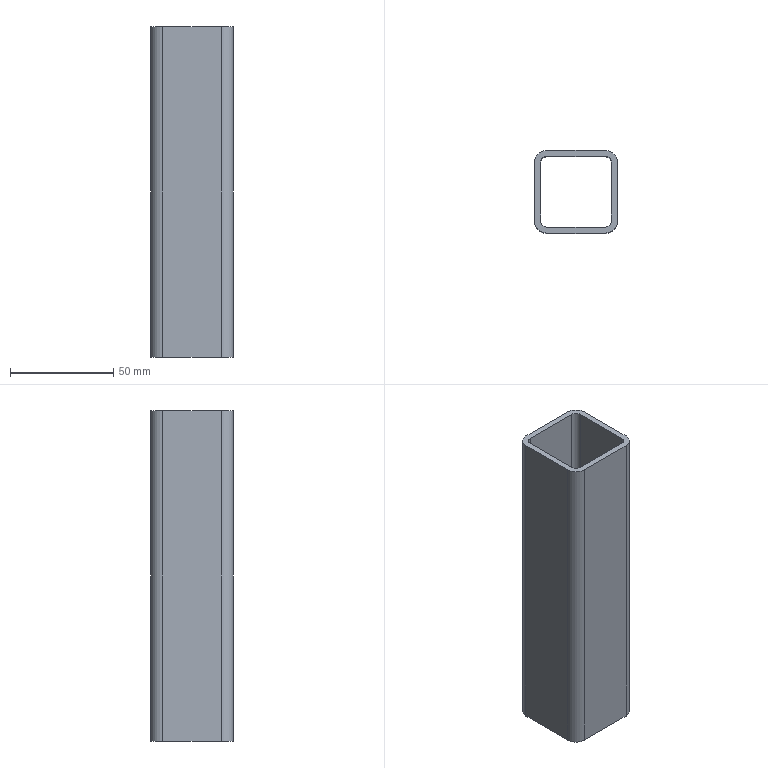Part | STEP file | DIN 59 410 - 40x40x2.9-200 | 1 solid | 18 faces | box 40 x 40 x 160 mm | volume 65392 mm3 | plane 10 | cylinder 8 | commonest cylinder face diameters 5.8 x4 11.6 x4
STEP:
#1=CARTESIAN_POINT('',(0.,0.,0.));
#2=DIRECTION('',(0.,0.,1.));
#3=DIRECTION('',(1.,0.,0.));
#4=AXIS2_PLACEMENT_3D('',#1,#2,#3);
#5=CARTESIAN_POINT('',(-14.2,-17.1,160.));
#6=VERTEX_POINT('',#5);
#7=CARTESIAN_POINT('',(14.2,-17.1,160.));
#8=VERTEX_POINT('',#7);
#9=CARTESIAN_POINT('',(7.1,-17.1,160.));
#10=DIRECTION('',(1.,0.,0.));
#11=VECTOR('',#10,1.);
#12=LINE('',#9,#11);
#13=CARTESIAN_POINT('',(14.2,-17.1,0.));
#14=DIRECTION('',(0.,-1.,0.));
#15=DIRECTION('',(0.,0.,-1.));
#16=AXIS2_PLACEMENT_3D('',#13,#14,#15);
#17=PLANE('',#16);
#18=CARTESIAN_POINT('',(-160.,-7.1));
#19=DIRECTION('',(0.,1.));
#20=VECTOR('',#19,1.);
#21=LINE('',#18,#20);
#22=(GEOMETRIC_REPRESENTATION_CONTEXT(2)PARAMETRIC_REPRESENTATION_CONTEXT()REPRESENTATION_CONTEXT('',''));
#23=DEFINITIONAL_REPRESENTATION('',(#21),#22);
#24=PCURVE('',#17,#23);
#25=CARTESIAN_POINT('',(0.,0.,160.));
#26=DIRECTION('',(0.,0.,1.));
#27=DIRECTION('',(1.,0.,0.));
#28=AXIS2_PLACEMENT_3D('',#25,#26,#27);
#29=PLANE('',#28);
#30=CARTESIAN_POINT('',(7.1,-17.1));
#31=DIRECTION('',(1.,0.));
#32=VECTOR('',#31,1.);
#33=LINE('',#30,#32);
#34=(GEOMETRIC_REPRESENTATION_CONTEXT(2)PARAMETRIC_REPRESENTATION_CONTEXT()REPRESENTATION_CONTEXT('',''));
#35=DEFINITIONAL_REPRESENTATION('',(#33),#34);
#36=PCURVE('',#29,#35);
#37=SURFACE_CURVE('',#12,(#24,#36),.PCURVE_S1.);
#38=EDGE_CURVE('',#6,#8,#37,.T.);
#39=ORIENTED_EDGE('',*,*,#38,.T.);
#40=CARTESIAN_POINT('',(14.2,-17.1,0.));
#41=VERTEX_POINT('',#40);
#42=CARTESIAN_POINT('',(14.2,-17.1,0.));
#43=DIRECTION('',(0.,0.,1.));
#44=VECTOR('',#43,1.);
#45=LINE('',#42,#44);
#46=CARTESIAN_POINT('',(0.,0.));
#47=DIRECTION('',(-1.,0.));
#48=VECTOR('',#47,1.);
#49=LINE('',#46,#48);
#50=(GEOMETRIC_REPRESENTATION_CONTEXT(2)PARAMETRIC_REPRESENTATION_CONTEXT()REPRESENTATION_CONTEXT('',''));
#51=DEFINITIONAL_REPRESENTATION('',(#49),#50);
#52=PCURVE('',#17,#51);
#53=CARTESIAN_POINT('',(14.2,-14.2,0.));
#54=DIRECTION('',(0.,0.,1.));
#55=DIRECTION('',(0.,1.,0.));
#56=AXIS2_PLACEMENT_3D('',#53,#54,#55);
#57=CYLINDRICAL_SURFACE('',#56,2.9);
#58=CARTESIAN_POINT('',(3.142,0.));
#59=DIRECTION('',(0.,1.));
#60=VECTOR('',#59,1.);
#61=LINE('',#58,#60);
#62=(GEOMETRIC_REPRESENTATION_CONTEXT(2)PARAMETRIC_REPRESENTATION_CONTEXT()REPRESENTATION_CONTEXT('',''));
#63=DEFINITIONAL_REPRESENTATION('',(#61),#62);
#64=PCURVE('',#57,#63);
#65=SURFACE_CURVE('',#45,(#52,#64),.PCURVE_S1.);
#66=EDGE_CURVE('',#41,#8,#65,.T.);
#67=ORIENTED_EDGE('',*,*,#66,.F.);
#68=CARTESIAN_POINT('',(-14.2,-17.1,0.));
#69=VERTEX_POINT('',#68);
#70=CARTESIAN_POINT('',(7.1,-17.1,0.));
#71=DIRECTION('',(1.,0.,0.));
#72=VECTOR('',#71,1.);
#73=LINE('',#70,#72);
#74=CARTESIAN_POINT('',(0.,-7.1));
#75=DIRECTION('',(0.,1.));
#76=VECTOR('',#75,1.);
#77=LINE('',#74,#76);
#78=(GEOMETRIC_REPRESENTATION_CONTEXT(2)PARAMETRIC_REPRESENTATION_CONTEXT()REPRESENTATION_CONTEXT('',''));
#79=DEFINITIONAL_REPRESENTATION('',(#77),#78);
#80=PCURVE('',#17,#79);
#81=CARTESIAN_POINT('',(0.,0.,0.));
#82=DIRECTION('',(0.,0.,1.));
#83=DIRECTION('',(1.,0.,0.));
#84=AXIS2_PLACEMENT_3D('',#81,#82,#83);
#85=PLANE('',#84);
#86=CARTESIAN_POINT('',(7.1,-17.1));
#87=DIRECTION('',(1.,0.));
#88=VECTOR('',#87,1.);
#89=LINE('',#86,#88);
#90=(GEOMETRIC_REPRESENTATION_CONTEXT(2)PARAMETRIC_REPRESENTATION_CONTEXT()REPRESENTATION_CONTEXT('',''));
#91=DEFINITIONAL_REPRESENTATION('',(#89),#90);
#92=PCURVE('',#85,#91);
#93=SURFACE_CURVE('',#73,(#80,#92),.PCURVE_S1.);
#94=EDGE_CURVE('',#69,#41,#93,.T.);
#95=ORIENTED_EDGE('',*,*,#94,.F.);
#96=CARTESIAN_POINT('',(-14.2,-17.1,0.));
#97=DIRECTION('',(0.,0.,1.));
#98=VECTOR('',#97,1.);
#99=LINE('',#96,#98);
#100=CARTESIAN_POINT('',(0.,-28.4));
#101=DIRECTION('',(-1.,0.));
#102=VECTOR('',#101,1.);
#103=LINE('',#100,#102);
#104=(GEOMETRIC_REPRESENTATION_CONTEXT(2)PARAMETRIC_REPRESENTATION_CONTEXT()REPRESENTATION_CONTEXT('',''));
#105=DEFINITIONAL_REPRESENTATION('',(#103),#104);
#106=PCURVE('',#17,#105);
#107=CARTESIAN_POINT('',(-14.2,-14.2,0.));
#108=DIRECTION('',(0.,0.,1.));
#109=DIRECTION('',(1.,0.,0.));
#110=AXIS2_PLACEMENT_3D('',#107,#108,#109);
#111=CYLINDRICAL_SURFACE('',#110,2.9);
#112=CARTESIAN_POINT('',(4.712,0.));
#113=DIRECTION('',(0.,1.));
#114=VECTOR('',#113,1.);
#115=LINE('',#112,#114);
#116=(GEOMETRIC_REPRESENTATION_CONTEXT(2)PARAMETRIC_REPRESENTATION_CONTEXT()REPRESENTATION_CONTEXT('',''));
#117=DEFINITIONAL_REPRESENTATION('',(#115),#116);
#118=PCURVE('',#111,#117);
#119=SURFACE_CURVE('',#99,(#106,#118),.PCURVE_S1.);
#120=EDGE_CURVE('',#69,#6,#119,.T.);
#121=ORIENTED_EDGE('',*,*,#120,.T.);
#122=EDGE_LOOP('',(#39,#67,#95,#121));
#123=FACE_BOUND('',#122,.T.);
#124=ADVANCED_FACE('',(#123),#17,.F.);
#125=ORIENTED_EDGE('',*,*,#66,.F.);
#126=CARTESIAN_POINT('',(17.1,-14.2,0.));
#127=VERTEX_POINT('',#126);
#128=CARTESIAN_POINT('',(14.2,-14.2,0.));
#129=DIRECTION('',(0.,0.,1.));
#130=DIRECTION('',(0.,1.,0.));
#131=AXIS2_PLACEMENT_3D('',#128,#129,#130);
#132=CIRCLE('',#131,2.9);
#133=CARTESIAN_POINT('',(0.,0.));
#134=DIRECTION('',(1.,0.));
#135=VECTOR('',#134,1.);
#136=LINE('',#133,#135);
#137=(GEOMETRIC_REPRESENTATION_CONTEXT(2)PARAMETRIC_REPRESENTATION_CONTEXT()REPRESENTATION_CONTEXT('',''));
#138=DEFINITIONAL_REPRESENTATION('',(#136),#137);
#139=PCURVE('',#57,#138);
#140=CARTESIAN_POINT('',(14.2,-14.2));
#141=DIRECTION('',(0.,1.));
#142=AXIS2_PLACEMENT_2D('',#140,#141);
#143=CIRCLE('',#142,2.9);
#144=(GEOMETRIC_REPRESENTATION_CONTEXT(2)PARAMETRIC_REPRESENTATION_CONTEXT()REPRESENTATION_CONTEXT('',''));
#145=DEFINITIONAL_REPRESENTATION('',(#143),#144);
#146=PCURVE('',#85,#145);
#147=SURFACE_CURVE('',#132,(#139,#146),.PCURVE_S1.);
#148=EDGE_CURVE('',#41,#127,#147,.T.);
#149=ORIENTED_EDGE('',*,*,#148,.T.);
#150=CARTESIAN_POINT('',(17.1,-14.2,160.));
#151=VERTEX_POINT('',#150);
#152=CARTESIAN_POINT('',(17.1,-14.2,0.));
#153=DIRECTION('',(0.,0.,1.));
#154=VECTOR('',#153,1.);
#155=LINE('',#152,#154);
#156=CARTESIAN_POINT('',(4.712,0.));
#157=DIRECTION('',(0.,1.));
#158=VECTOR('',#157,1.);
#159=LINE('',#156,#158);
#160=(GEOMETRIC_REPRESENTATION_CONTEXT(2)PARAMETRIC_REPRESENTATION_CONTEXT()REPRESENTATION_CONTEXT('',''));
#161=DEFINITIONAL_REPRESENTATION('',(#159),#160);
#162=PCURVE('',#57,#161);
#163=CARTESIAN_POINT('',(17.1,14.2,0.));
#164=DIRECTION('',(1.,0.,0.));
#165=DIRECTION('',(0.,0.,-1.));
#166=AXIS2_PLACEMENT_3D('',#163,#164,#165);
#167=PLANE('',#166);
#168=CARTESIAN_POINT('',(0.,-28.4));
#169=DIRECTION('',(-1.,0.));
#170=VECTOR('',#169,1.);
#171=LINE('',#168,#170);
#172=(GEOMETRIC_REPRESENTATION_CONTEXT(2)PARAMETRIC_REPRESENTATION_CONTEXT()REPRESENTATION_CONTEXT('',''));
#173=DEFINITIONAL_REPRESENTATION('',(#171),#172);
#174=PCURVE('',#167,#173);
#175=SURFACE_CURVE('',#155,(#162,#174),.PCURVE_S1.);
#176=EDGE_CURVE('',#127,#151,#175,.T.);
#177=ORIENTED_EDGE('',*,*,#176,.T.);
#178=CARTESIAN_POINT('',(14.2,-14.2,160.));
#179=DIRECTION('',(0.,0.,1.));
#180=DIRECTION('',(0.,1.,0.));
#181=AXIS2_PLACEMENT_3D('',#178,#179,#180);
#182=CIRCLE('',#181,2.9);
#183=CARTESIAN_POINT('',(0.,160.));
#184=DIRECTION('',(1.,0.));
#185=VECTOR('',#184,1.);
#186=LINE('',#183,#185);
#187=(GEOMETRIC_REPRESENTATION_CONTEXT(2)PARAMETRIC_REPRESENTATION_CONTEXT()REPRESENTATION_CONTEXT('',''));
#188=DEFINITIONAL_REPRESENTATION('',(#186),#187);
#189=PCURVE('',#57,#188);
#190=CARTESIAN_POINT('',(14.2,-14.2));
#191=DIRECTION('',(0.,1.));
#192=AXIS2_PLACEMENT_2D('',#190,#191);
#193=CIRCLE('',#192,2.9);
#194=(GEOMETRIC_REPRESENTATION_CONTEXT(2)PARAMETRIC_REPRESENTATION_CONTEXT()REPRESENTATION_CONTEXT('',''));
#195=DEFINITIONAL_REPRESENTATION('',(#193),#194);
#196=PCURVE('',#29,#195);
#197=SURFACE_CURVE('',#182,(#189,#196),.PCURVE_S1.);
#198=EDGE_CURVE('',#8,#151,#197,.T.);
#199=ORIENTED_EDGE('',*,*,#198,.F.);
#200=EDGE_LOOP('',(#125,#149,#177,#199));
#201=FACE_BOUND('',#200,.F.);
#202=ADVANCED_FACE('',(#201),#57,.F.);
#203=CARTESIAN_POINT('',(17.1,14.2,160.));
#204=VERTEX_POINT('',#203);
#205=CARTESIAN_POINT('',(17.1,7.1,160.));
#206=DIRECTION('',(0.,1.,0.));
#207=VECTOR('',#206,1.);
#208=LINE('',#205,#207);
#209=CARTESIAN_POINT('',(-160.,-7.1));
#210=DIRECTION('',(0.,1.));
#211=VECTOR('',#210,1.);
#212=LINE('',#209,#211);
#213=(GEOMETRIC_REPRESENTATION_CONTEXT(2)PARAMETRIC_REPRESENTATION_CONTEXT()REPRESENTATION_CONTEXT('',''));
#214=DEFINITIONAL_REPRESENTATION('',(#212),#213);
#215=PCURVE('',#167,#214);
#216=CARTESIAN_POINT('',(17.1,7.1));
#217=DIRECTION('',(0.,1.));
#218=VECTOR('',#217,1.);
#219=LINE('',#216,#218);
#220=(GEOMETRIC_REPRESENTATION_CONTEXT(2)PARAMETRIC_REPRESENTATION_CONTEXT()REPRESENTATION_CONTEXT('',''));
#221=DEFINITIONAL_REPRESENTATION('',(#219),#220);
#222=PCURVE('',#29,#221);
#223=SURFACE_CURVE('',#208,(#215,#222),.PCURVE_S1.);
#224=EDGE_CURVE('',#151,#204,#223,.T.);
#225=ORIENTED_EDGE('',*,*,#224,.T.);
#226=CARTESIAN_POINT('',(17.1,14.2,0.));
#227=VERTEX_POINT('',#226);
#228=CARTESIAN_POINT('',(17.1,14.2,0.));
#229=DIRECTION('',(0.,0.,1.));
#230=VECTOR('',#229,1.);
#231=LINE('',#228,#230);
#232=CARTESIAN_POINT('',(0.,0.));
#233=DIRECTION('',(-1.,0.));
#234=VECTOR('',#233,1.);
#235=LINE('',#232,#234);
#236=(GEOMETRIC_REPRESENTATION_CONTEXT(2)PARAMETRIC_REPRESENTATION_CONTEXT()REPRESENTATION_CONTEXT('',''));
#237=DEFINITIONAL_REPRESENTATION('',(#235),#236);
#238=PCURVE('',#167,#237);
#239=CARTESIAN_POINT('',(14.2,14.2,0.));
#240=DIRECTION('',(0.,0.,1.));
#241=DIRECTION('',(-1.,0.,0.));
#242=AXIS2_PLACEMENT_3D('',#239,#240,#241);
#243=CYLINDRICAL_SURFACE('',#242,2.9);
#244=CARTESIAN_POINT('',(3.142,0.));
#245=DIRECTION('',(0.,1.));
#246=VECTOR('',#245,1.);
#247=LINE('',#244,#246);
#248=(GEOMETRIC_REPRESENTATION_CONTEXT(2)PARAMETRIC_REPRESENTATION_CONTEXT()REPRESENTATION_CONTEXT('',''));
#249=DEFINITIONAL_REPRESENTATION('',(#247),#248);
#250=PCURVE('',#243,#249);
#251=SURFACE_CURVE('',#231,(#238,#250),.PCURVE_S1.);
#252=EDGE_CURVE('',#227,#204,#251,.T.);
#253=ORIENTED_EDGE('',*,*,#252,.F.);
#254=CARTESIAN_POINT('',(17.1,7.1,0.));
#255=DIRECTION('',(0.,1.,0.));
#256=VECTOR('',#255,1.);
#257=LINE('',#254,#256);
#258=CARTESIAN_POINT('',(0.,-7.1));
#259=DIRECTION('',(0.,1.));
#260=VECTOR('',#259,1.);
#261=LINE('',#258,#260);
#262=(GEOMETRIC_REPRESENTATION_CONTEXT(2)PARAMETRIC_REPRESENTATION_CONTEXT()REPRESENTATION_CONTEXT('',''));
#263=DEFINITIONAL_REPRESENTATION('',(#261),#262);
#264=PCURVE('',#167,#263);
#265=CARTESIAN_POINT('',(17.1,7.1));
#266=DIRECTION('',(0.,1.));
#267=VECTOR('',#266,1.);
#268=LINE('',#265,#267);
#269=(GEOMETRIC_REPRESENTATION_CONTEXT(2)PARAMETRIC_REPRESENTATION_CONTEXT()REPRESENTATION_CONTEXT('',''));
#270=DEFINITIONAL_REPRESENTATION('',(#268),#269);
#271=PCURVE('',#85,#270);
#272=SURFACE_CURVE('',#257,(#264,#271),.PCURVE_S1.);
#273=EDGE_CURVE('',#127,#227,#272,.T.);
#274=ORIENTED_EDGE('',*,*,#273,.F.);
#275=ORIENTED_EDGE('',*,*,#176,.T.);
#276=EDGE_LOOP('',(#225,#253,#274,#275));
#277=FACE_BOUND('',#276,.T.);
#278=ADVANCED_FACE('',(#277),#167,.F.);
#279=ORIENTED_EDGE('',*,*,#252,.F.);
#280=CARTESIAN_POINT('',(14.2,17.1,0.));
#281=VERTEX_POINT('',#280);
#282=CARTESIAN_POINT('',(14.2,14.2,0.));
#283=DIRECTION('',(0.,0.,1.));
#284=DIRECTION('',(-1.,0.,0.));
#285=AXIS2_PLACEMENT_3D('',#282,#283,#284);
#286=CIRCLE('',#285,2.9);
#287=CARTESIAN_POINT('',(0.,0.));
#288=DIRECTION('',(1.,0.));
#289=VECTOR('',#288,1.);
#290=LINE('',#287,#289);
#291=(GEOMETRIC_REPRESENTATION_CONTEXT(2)PARAMETRIC_REPRESENTATION_CONTEXT()REPRESENTATION_CONTEXT('',''));
#292=DEFINITIONAL_REPRESENTATION('',(#290),#291);
#293=PCURVE('',#243,#292);
#294=CARTESIAN_POINT('',(14.2,14.2));
#295=DIRECTION('',(-1.,0.));
#296=AXIS2_PLACEMENT_2D('',#294,#295);
#297=CIRCLE('',#296,2.9);
#298=(GEOMETRIC_REPRESENTATION_CONTEXT(2)PARAMETRIC_REPRESENTATION_CONTEXT()REPRESENTATION_CONTEXT('',''));
#299=DEFINITIONAL_REPRESENTATION('',(#297),#298);
#300=PCURVE('',#85,#299);
#301=SURFACE_CURVE('',#286,(#293,#300),.PCURVE_S1.);
#302=EDGE_CURVE('',#227,#281,#301,.T.);
#303=ORIENTED_EDGE('',*,*,#302,.T.);
#304=CARTESIAN_POINT('',(14.2,17.1,160.));
#305=VERTEX_POINT('',#304);
#306=CARTESIAN_POINT('',(14.2,17.1,0.));
#307=DIRECTION('',(0.,0.,1.));
#308=VECTOR('',#307,1.);
#309=LINE('',#306,#308);
#310=CARTESIAN_POINT('',(4.712,0.));
#311=DIRECTION('',(0.,1.));
#312=VECTOR('',#311,1.);
#313=LINE('',#310,#312);
#314=(GEOMETRIC_REPRESENTATION_CONTEXT(2)PARAMETRIC_REPRESENTATION_CONTEXT()REPRESENTATION_CONTEXT('',''));
#315=DEFINITIONAL_REPRESENTATION('',(#313),#314);
#316=PCURVE('',#243,#315);
#317=CARTESIAN_POINT('',(-14.2,17.1,0.));
#318=DIRECTION('',(0.,1.,0.));
#319=DIRECTION('',(0.,0.,1.));
#320=AXIS2_PLACEMENT_3D('',#317,#318,#319);
#321=PLANE('',#320);
#322=CARTESIAN_POINT('',(0.,28.4));
#323=DIRECTION('',(1.,0.));
#324=VECTOR('',#323,1.);
#325=LINE('',#322,#324);
#326=(GEOMETRIC_REPRESENTATION_CONTEXT(2)PARAMETRIC_REPRESENTATION_CONTEXT()REPRESENTATION_CONTEXT('',''));
#327=DEFINITIONAL_REPRESENTATION('',(#325),#326);
#328=PCURVE('',#321,#327);
#329=SURFACE_CURVE('',#309,(#316,#328),.PCURVE_S1.);
#330=EDGE_CURVE('',#281,#305,#329,.T.);
#331=ORIENTED_EDGE('',*,*,#330,.T.);
#332=CARTESIAN_POINT('',(14.2,14.2,160.));
#333=DIRECTION('',(0.,0.,1.));
#334=DIRECTION('',(-1.,0.,0.));
#335=AXIS2_PLACEMENT_3D('',#332,#333,#334);
#336=CIRCLE('',#335,2.9);
#337=CARTESIAN_POINT('',(0.,160.));
#338=DIRECTION('',(1.,0.));
#339=VECTOR('',#338,1.);
#340=LINE('',#337,#339);
#341=(GEOMETRIC_REPRESENTATION_CONTEXT(2)PARAMETRIC_REPRESENTATION_CONTEXT()REPRESENTATION_CONTEXT('',''));
#342=DEFINITIONAL_REPRESENTATION('',(#340),#341);
#343=PCURVE('',#243,#342);
#344=CARTESIAN_POINT('',(14.2,14.2));
#345=DIRECTION('',(-1.,0.));
#346=AXIS2_PLACEMENT_2D('',#344,#345);
#347=CIRCLE('',#346,2.9);
#348=(GEOMETRIC_REPRESENTATION_CONTEXT(2)PARAMETRIC_REPRESENTATION_CONTEXT()REPRESENTATION_CONTEXT('',''));
#349=DEFINITIONAL_REPRESENTATION('',(#347),#348);
#350=PCURVE('',#29,#349);
#351=SURFACE_CURVE('',#336,(#343,#350),.PCURVE_S1.);
#352=EDGE_CURVE('',#204,#305,#351,.T.);
#353=ORIENTED_EDGE('',*,*,#352,.F.);
#354=EDGE_LOOP('',(#279,#303,#331,#353));
#355=FACE_BOUND('',#354,.F.);
#356=ADVANCED_FACE('',(#355),#243,.F.);
#357=CARTESIAN_POINT('',(14.2,-20.,160.));
#358=VERTEX_POINT('',#357);
#359=CARTESIAN_POINT('',(-14.2,-20.,160.));
#360=VERTEX_POINT('',#359);
#361=CARTESIAN_POINT('',(7.1,-20.,160.));
#362=DIRECTION('',(-1.,0.,0.));
#363=VECTOR('',#362,1.);
#364=LINE('',#361,#363);
#365=CARTESIAN_POINT('',(14.2,-20.,0.));
#366=DIRECTION('',(0.,-1.,0.));
#367=DIRECTION('',(0.,0.,-1.));
#368=AXIS2_PLACEMENT_3D('',#365,#366,#367);
#369=PLANE('',#368);
#370=CARTESIAN_POINT('',(-160.,-7.1));
#371=DIRECTION('',(0.,-1.));
#372=VECTOR('',#371,1.);
#373=LINE('',#370,#372);
#374=(GEOMETRIC_REPRESENTATION_CONTEXT(2)PARAMETRIC_REPRESENTATION_CONTEXT()REPRESENTATION_CONTEXT('',''));
#375=DEFINITIONAL_REPRESENTATION('',(#373),#374);
#376=PCURVE('',#369,#375);
#377=CARTESIAN_POINT('',(7.1,-20.));
#378=DIRECTION('',(-1.,0.));
#379=VECTOR('',#378,1.);
#380=LINE('',#377,#379);
#381=(GEOMETRIC_REPRESENTATION_CONTEXT(2)PARAMETRIC_REPRESENTATION_CONTEXT()REPRESENTATION_CONTEXT('',''));
#382=DEFINITIONAL_REPRESENTATION('',(#380),#381);
#383=PCURVE('',#29,#382);
#384=SURFACE_CURVE('',#364,(#376,#383),.PCURVE_S1.);
#385=EDGE_CURVE('',#358,#360,#384,.T.);
#386=ORIENTED_EDGE('',*,*,#385,.T.);
#387=CARTESIAN_POINT('',(-14.2,-20.,0.));
#388=VERTEX_POINT('',#387);
#389=CARTESIAN_POINT('',(-14.2,-20.,0.));
#390=DIRECTION('',(0.,0.,1.));
#391=VECTOR('',#390,1.);
#392=LINE('',#389,#391);
#393=CARTESIAN_POINT('',(0.,-28.4));
#394=DIRECTION('',(-1.,0.));
#395=VECTOR('',#394,1.);
#396=LINE('',#393,#395);
#397=(GEOMETRIC_REPRESENTATION_CONTEXT(2)PARAMETRIC_REPRESENTATION_CONTEXT()REPRESENTATION_CONTEXT('',''));
#398=DEFINITIONAL_REPRESENTATION('',(#396),#397);
#399=PCURVE('',#369,#398);
#400=CARTESIAN_POINT('',(-14.2,-14.2,0.));
#401=DIRECTION('',(0.,0.,1.));
#402=DIRECTION('',(1.,0.,0.));
#403=AXIS2_PLACEMENT_3D('',#400,#401,#402);
#404=CYLINDRICAL_SURFACE('',#403,5.8);
#405=CARTESIAN_POINT('',(4.712,0.));
#406=DIRECTION('',(0.,1.));
#407=VECTOR('',#406,1.);
#408=LINE('',#405,#407);
#409=(GEOMETRIC_REPRESENTATION_CONTEXT(2)PARAMETRIC_REPRESENTATION_CONTEXT()REPRESENTATION_CONTEXT('',''));
#410=DEFINITIONAL_REPRESENTATION('',(#408),#409);
#411=PCURVE('',#404,#410);
#412=SURFACE_CURVE('',#392,(#399,#411),.PCURVE_S1.);
#413=EDGE_CURVE('',#388,#360,#412,.T.);
#414=ORIENTED_EDGE('',*,*,#413,.F.);
#415=CARTESIAN_POINT('',(14.2,-20.,0.));
#416=VERTEX_POINT('',#415);
#417=CARTESIAN_POINT('',(7.1,-20.,0.));
#418=DIRECTION('',(-1.,0.,0.));
#419=VECTOR('',#418,1.);
#420=LINE('',#417,#419);
#421=CARTESIAN_POINT('',(0.,-7.1));
#422=DIRECTION('',(0.,-1.));
#423=VECTOR('',#422,1.);
#424=LINE('',#421,#423);
#425=(GEOMETRIC_REPRESENTATION_CONTEXT(2)PARAMETRIC_REPRESENTATION_CONTEXT()REPRESENTATION_CONTEXT('',''));
#426=DEFINITIONAL_REPRESENTATION('',(#424),#425);
#427=PCURVE('',#369,#426);
#428=CARTESIAN_POINT('',(7.1,-20.));
#429=DIRECTION('',(-1.,0.));
#430=VECTOR('',#429,1.);
#431=LINE('',#428,#430);
#432=(GEOMETRIC_REPRESENTATION_CONTEXT(2)PARAMETRIC_REPRESENTATION_CONTEXT()REPRESENTATION_CONTEXT('',''));
#433=DEFINITIONAL_REPRESENTATION('',(#431),#432);
#434=PCURVE('',#85,#433);
#435=SURFACE_CURVE('',#420,(#427,#434),.PCURVE_S1.);
#436=EDGE_CURVE('',#416,#388,#435,.T.);
#437=ORIENTED_EDGE('',*,*,#436,.F.);
#438=CARTESIAN_POINT('',(14.2,-20.,0.));
#439=DIRECTION('',(0.,0.,1.));
#440=VECTOR('',#439,1.);
#441=LINE('',#438,#440);
#442=CARTESIAN_POINT('',(0.,0.));
#443=DIRECTION('',(-1.,0.));
#444=VECTOR('',#443,1.);
#445=LINE('',#442,#444);
#446=(GEOMETRIC_REPRESENTATION_CONTEXT(2)PARAMETRIC_REPRESENTATION_CONTEXT()REPRESENTATION_CONTEXT('',''));
#447=DEFINITIONAL_REPRESENTATION('',(#445),#446);
#448=PCURVE('',#369,#447);
#449=CARTESIAN_POINT('',(14.2,-14.2,0.));
#450=DIRECTION('',(0.,0.,1.));
#451=DIRECTION('',(0.,1.,0.));
#452=AXIS2_PLACEMENT_3D('',#449,#450,#451);
#453=CYLINDRICAL_SURFACE('',#452,5.8);
#454=CARTESIAN_POINT('',(3.142,0.));
#455=DIRECTION('',(0.,1.));
#456=VECTOR('',#455,1.);
#457=LINE('',#454,#456);
#458=(GEOMETRIC_REPRESENTATION_CONTEXT(2)PARAMETRIC_REPRESENTATION_CONTEXT()REPRESENTATION_CONTEXT('',''));
#459=DEFINITIONAL_REPRESENTATION('',(#457),#458);
#460=PCURVE('',#453,#459);
#461=SURFACE_CURVE('',#441,(#448,#460),.PCURVE_S1.);
#462=EDGE_CURVE('',#416,#358,#461,.T.);
#463=ORIENTED_EDGE('',*,*,#462,.T.);
#464=EDGE_LOOP('',(#386,#414,#437,#463));
#465=FACE_BOUND('',#464,.T.);
#466=ADVANCED_FACE('',(#465),#369,.T.);
#467=CARTESIAN_POINT('',(-20.,-14.2,160.));
#468=VERTEX_POINT('',#467);
#469=CARTESIAN_POINT('',(-14.2,-14.2,160.));
#470=DIRECTION('',(0.,0.,-1.));
#471=DIRECTION('',(1.,0.,0.));
#472=AXIS2_PLACEMENT_3D('',#469,#470,#471);
#473=CIRCLE('',#472,5.8);
#474=CARTESIAN_POINT('',(6.283,160.));
#475=DIRECTION('',(-1.,0.));
#476=VECTOR('',#475,1.);
#477=LINE('',#474,#476);
#478=(GEOMETRIC_REPRESENTATION_CONTEXT(2)PARAMETRIC_REPRESENTATION_CONTEXT()REPRESENTATION_CONTEXT('',''));
#479=DEFINITIONAL_REPRESENTATION('',(#477),#478);
#480=PCURVE('',#404,#479);
#481=CARTESIAN_POINT('',(-8.4,-14.2));
#482=CARTESIAN_POINT('',(-8.4,-24.246));
#483=CARTESIAN_POINT('',(-17.1,-19.223));
#484=CARTESIAN_POINT('',(-25.8,-14.2));
#485=CARTESIAN_POINT('',(-17.1,-9.177));
#486=CARTESIAN_POINT('',(-8.4,-4.154));
#487=CARTESIAN_POINT('',(-8.4,-14.2));
#488=(BOUNDED_CURVE()B_SPLINE_CURVE(2,(#481,#482,#483,#484,#485,#486,#487),.UNSPECIFIED.,.T.,.F.)B_SPLINE_CURVE_WITH_KNOTS((1,2,2,2,2,1),(-2.094,0.,2.094,4.189,6.283,8.378),.UNSPECIFIED.)CURVE()GEOMETRIC_REPRESENTATION_ITEM()RATIONAL_B_SPLINE_CURVE((1.,0.5,1.,0.5,1.,0.5,1.))REPRESENTATION_ITEM(''));
#489=(GEOMETRIC_REPRESENTATION_CONTEXT(2)PARAMETRIC_REPRESENTATION_CONTEXT()REPRESENTATION_CONTEXT('',''));
#490=DEFINITIONAL_REPRESENTATION('',(#488),#489);
#491=PCURVE('',#29,#490);
#492=SURFACE_CURVE('',#473,(#480,#491),.PCURVE_S1.);
#493=EDGE_CURVE('',#360,#468,#492,.T.);
#494=ORIENTED_EDGE('',*,*,#493,.T.);
#495=CARTESIAN_POINT('',(-20.,-14.2,0.));
#496=VERTEX_POINT('',#495);
#497=CARTESIAN_POINT('',(-20.,-14.2,0.));
#498=DIRECTION('',(0.,0.,1.));
#499=VECTOR('',#498,1.);
#500=LINE('',#497,#499);
#501=CARTESIAN_POINT('',(3.142,0.));
#502=DIRECTION('',(0.,1.));
#503=VECTOR('',#502,1.);
#504=LINE('',#501,#503);
#505=(GEOMETRIC_REPRESENTATION_CONTEXT(2)PARAMETRIC_REPRESENTATION_CONTEXT()REPRESENTATION_CONTEXT('',''));
#506=DEFINITIONAL_REPRESENTATION('',(#504),#505);
#507=PCURVE('',#404,#506);
#508=CARTESIAN_POINT('',(-20.,-14.2,0.));
#509=DIRECTION('',(-1.,0.,0.));
#510=DIRECTION('',(0.,0.,1.));
#511=AXIS2_PLACEMENT_3D('',#508,#509,#510);
#512=PLANE('',#511);
#513=CARTESIAN_POINT('',(0.,0.));
#514=DIRECTION('',(1.,0.));
#515=VECTOR('',#514,1.);
#516=LINE('',#513,#515);
#517=(GEOMETRIC_REPRESENTATION_CONTEXT(2)PARAMETRIC_REPRESENTATION_CONTEXT()REPRESENTATION_CONTEXT('',''));
#518=DEFINITIONAL_REPRESENTATION('',(#516),#517);
#519=PCURVE('',#512,#518);
#520=SURFACE_CURVE('',#500,(#507,#519),.PCURVE_S1.);
#521=EDGE_CURVE('',#496,#468,#520,.T.);
#522=ORIENTED_EDGE('',*,*,#521,.F.);
#523=CARTESIAN_POINT('',(-14.2,-14.2,0.));
#524=DIRECTION('',(0.,0.,-1.));
#525=DIRECTION('',(1.,0.,0.));
#526=AXIS2_PLACEMENT_3D('',#523,#524,#525);
#527=CIRCLE('',#526,5.8);
#528=CARTESIAN_POINT('',(6.283,0.));
#529=DIRECTION('',(-1.,0.));
#530=VECTOR('',#529,1.);
#531=LINE('',#528,#530);
#532=(GEOMETRIC_REPRESENTATION_CONTEXT(2)PARAMETRIC_REPRESENTATION_CONTEXT()REPRESENTATION_CONTEXT('',''));
#533=DEFINITIONAL_REPRESENTATION('',(#531),#532);
#534=PCURVE('',#404,#533);
#535=CARTESIAN_POINT('',(-8.4,-14.2));
#536=CARTESIAN_POINT('',(-8.4,-24.246));
#537=CARTESIAN_POINT('',(-17.1,-19.223));
#538=CARTESIAN_POINT('',(-25.8,-14.2));
#539=CARTESIAN_POINT('',(-17.1,-9.177));
#540=CARTESIAN_POINT('',(-8.4,-4.154));
#541=CARTESIAN_POINT('',(-8.4,-14.2));
#542=(BOUNDED_CURVE()B_SPLINE_CURVE(2,(#535,#536,#537,#538,#539,#540,#541),.UNSPECIFIED.,.T.,.F.)B_SPLINE_CURVE_WITH_KNOTS((1,2,2,2,2,1),(-2.094,0.,2.094,4.189,6.283,8.378),.UNSPECIFIED.)CURVE()GEOMETRIC_REPRESENTATION_ITEM()RATIONAL_B_SPLINE_CURVE((1.,0.5,1.,0.5,1.,0.5,1.))REPRESENTATION_ITEM(''));
#543=(GEOMETRIC_REPRESENTATION_CONTEXT(2)PARAMETRIC_REPRESENTATION_CONTEXT()REPRESENTATION_CONTEXT('',''));
#544=DEFINITIONAL_REPRESENTATION('',(#542),#543);
#545=PCURVE('',#85,#544);
#546=SURFACE_CURVE('',#527,(#534,#545),.PCURVE_S1.);
#547=EDGE_CURVE('',#388,#496,#546,.T.);
#548=ORIENTED_EDGE('',*,*,#547,.F.);
#549=ORIENTED_EDGE('',*,*,#413,.T.);
#550=EDGE_LOOP('',(#494,#522,#548,#549));
#551=FACE_BOUND('',#550,.T.);
#552=ADVANCED_FACE('',(#551),#404,.T.);
#553=CARTESIAN_POINT('',(-20.,14.2,160.));
#554=VERTEX_POINT('',#553);
#555=CARTESIAN_POINT('',(-20.,-7.1,160.));
#556=DIRECTION('',(0.,1.,0.));
#557=VECTOR('',#556,1.);
#558=LINE('',#555,#557);
#559=CARTESIAN_POINT('',(160.,7.1));
#560=DIRECTION('',(0.,1.));
#561=VECTOR('',#560,1.);
#562=LINE('',#559,#561);
#563=(GEOMETRIC_REPRESENTATION_CONTEXT(2)PARAMETRIC_REPRESENTATION_CONTEXT()REPRESENTATION_CONTEXT('',''));
#564=DEFINITIONAL_REPRESENTATION('',(#562),#563);
#565=PCURVE('',#512,#564);
#566=CARTESIAN_POINT('',(-20.,-7.1));
#567=DIRECTION('',(0.,1.));
#568=VECTOR('',#567,1.);
#569=LINE('',#566,#568);
#570=(GEOMETRIC_REPRESENTATION_CONTEXT(2)PARAMETRIC_REPRESENTATION_CONTEXT()REPRESENTATION_CONTEXT('',''));
#571=DEFINITIONAL_REPRESENTATION('',(#569),#570);
#572=PCURVE('',#29,#571);
#573=SURFACE_CURVE('',#558,(#565,#572),.PCURVE_S1.);
#574=EDGE_CURVE('',#468,#554,#573,.T.);
#575=ORIENTED_EDGE('',*,*,#574,.T.);
#576=CARTESIAN_POINT('',(-20.,14.2,0.));
#577=VERTEX_POINT('',#576);
#578=CARTESIAN_POINT('',(-20.,14.2,0.));
#579=DIRECTION('',(0.,0.,1.));
#580=VECTOR('',#579,1.);
#581=LINE('',#578,#580);
#582=CARTESIAN_POINT('',(0.,28.4));
#583=DIRECTION('',(1.,0.));
#584=VECTOR('',#583,1.);
#585=LINE('',#582,#584);
#586=(GEOMETRIC_REPRESENTATION_CONTEXT(2)PARAMETRIC_REPRESENTATION_CONTEXT()REPRESENTATION_CONTEXT('',''));
#587=DEFINITIONAL_REPRESENTATION('',(#585),#586);
#588=PCURVE('',#512,#587);
#589=CARTESIAN_POINT('',(-14.2,14.2,0.));
#590=DIRECTION('',(0.,0.,1.));
#591=DIRECTION('',(0.,-1.,0.));
#592=AXIS2_PLACEMENT_3D('',#589,#590,#591);
#593=CYLINDRICAL_SURFACE('',#592,5.8);
#594=CARTESIAN_POINT('',(4.712,0.));
#595=DIRECTION('',(0.,1.));
#596=VECTOR('',#595,1.);
#597=LINE('',#594,#596);
#598=(GEOMETRIC_REPRESENTATION_CONTEXT(2)PARAMETRIC_REPRESENTATION_CONTEXT()REPRESENTATION_CONTEXT('',''));
#599=DEFINITIONAL_REPRESENTATION('',(#597),#598);
#600=PCURVE('',#593,#599);
#601=SURFACE_CURVE('',#581,(#588,#600),.PCURVE_S1.);
#602=EDGE_CURVE('',#577,#554,#601,.T.);
#603=ORIENTED_EDGE('',*,*,#602,.F.);
#604=CARTESIAN_POINT('',(-20.,-7.1,0.));
#605=DIRECTION('',(0.,1.,0.));
#606=VECTOR('',#605,1.);
#607=LINE('',#604,#606);
#608=CARTESIAN_POINT('',(0.,7.1));
#609=DIRECTION('',(0.,1.));
#610=VECTOR('',#609,1.);
#611=LINE('',#608,#610);
#612=(GEOMETRIC_REPRESENTATION_CONTEXT(2)PARAMETRIC_REPRESENTATION_CONTEXT()REPRESENTATION_CONTEXT('',''));
#613=DEFINITIONAL_REPRESENTATION('',(#611),#612);
#614=PCURVE('',#512,#613);
#615=CARTESIAN_POINT('',(-20.,-7.1));
#616=DIRECTION('',(0.,1.));
#617=VECTOR('',#616,1.);
#618=LINE('',#615,#617);
#619=(GEOMETRIC_REPRESENTATION_CONTEXT(2)PARAMETRIC_REPRESENTATION_CONTEXT()REPRESENTATION_CONTEXT('',''));
#620=DEFINITIONAL_REPRESENTATION('',(#618),#619);
#621=PCURVE('',#85,#620);
#622=SURFACE_CURVE('',#607,(#614,#621),.PCURVE_S1.);
#623=EDGE_CURVE('',#496,#577,#622,.T.);
#624=ORIENTED_EDGE('',*,*,#623,.F.);
#625=ORIENTED_EDGE('',*,*,#521,.T.);
#626=EDGE_LOOP('',(#575,#603,#624,#625));
#627=FACE_BOUND('',#626,.T.);
#628=ADVANCED_FACE('',(#627),#512,.T.);
#629=CARTESIAN_POINT('',(-14.2,20.,160.));
#630=VERTEX_POINT('',#629);
#631=CARTESIAN_POINT('',(-14.2,14.2,160.));
#632=DIRECTION('',(0.,0.,-1.));
#633=DIRECTION('',(0.,-1.,0.));
#634=AXIS2_PLACEMENT_3D('',#631,#632,#633);
#635=CIRCLE('',#634,5.8);
#636=CARTESIAN_POINT('',(6.283,160.));
#637=DIRECTION('',(-1.,0.));
#638=VECTOR('',#637,1.);
#639=LINE('',#636,#638);
#640=(GEOMETRIC_REPRESENTATION_CONTEXT(2)PARAMETRIC_REPRESENTATION_CONTEXT()REPRESENTATION_CONTEXT('',''));
#641=DEFINITIONAL_REPRESENTATION('',(#639),#640);
#642=PCURVE('',#593,#641);
#643=CARTESIAN_POINT('',(-14.2,8.4));
#644=CARTESIAN_POINT('',(-24.246,8.4));
#645=CARTESIAN_POINT('',(-19.223,17.1));
#646=CARTESIAN_POINT('',(-14.2,25.8));
#647=CARTESIAN_POINT('',(-9.177,17.1));
#648=CARTESIAN_POINT('',(-4.154,8.4));
#649=CARTESIAN_POINT('',(-14.2,8.4));
#650=(BOUNDED_CURVE()B_SPLINE_CURVE(2,(#643,#644,#645,#646,#647,#648,#649),.UNSPECIFIED.,.T.,.F.)B_SPLINE_CURVE_WITH_KNOTS((1,2,2,2,2,1),(-2.094,0.,2.094,4.189,6.283,8.378),.UNSPECIFIED.)CURVE()GEOMETRIC_REPRESENTATION_ITEM()RATIONAL_B_SPLINE_CURVE((1.,0.5,1.,0.5,1.,0.5,1.))REPRESENTATION_ITEM(''));
#651=(GEOMETRIC_REPRESENTATION_CONTEXT(2)PARAMETRIC_REPRESENTATION_CONTEXT()REPRESENTATION_CONTEXT('',''));
#652=DEFINITIONAL_REPRESENTATION('',(#650),#651);
#653=PCURVE('',#29,#652);
#654=SURFACE_CURVE('',#635,(#642,#653),.PCURVE_S1.);
#655=EDGE_CURVE('',#554,#630,#654,.T.);
#656=ORIENTED_EDGE('',*,*,#655,.T.);
#657=CARTESIAN_POINT('',(-14.2,20.,0.));
#658=VERTEX_POINT('',#657);
#659=CARTESIAN_POINT('',(-14.2,20.,0.));
#660=DIRECTION('',(0.,0.,1.));
#661=VECTOR('',#660,1.);
#662=LINE('',#659,#661);
#663=CARTESIAN_POINT('',(3.142,0.));
#664=DIRECTION('',(0.,1.));
#665=VECTOR('',#664,1.);
#666=LINE('',#663,#665);
#667=(GEOMETRIC_REPRESENTATION_CONTEXT(2)PARAMETRIC_REPRESENTATION_CONTEXT()REPRESENTATION_CONTEXT('',''));
#668=DEFINITIONAL_REPRESENTATION('',(#666),#667);
#669=PCURVE('',#593,#668);
#670=CARTESIAN_POINT('',(-14.2,20.,0.));
#671=DIRECTION('',(0.,1.,0.));
#672=DIRECTION('',(0.,0.,1.));
#673=AXIS2_PLACEMENT_3D('',#670,#671,#672);
#674=PLANE('',#673);
#675=CARTESIAN_POINT('',(0.,0.));
#676=DIRECTION('',(1.,0.));
#677=VECTOR('',#676,1.);
#678=LINE('',#675,#677);
#679=(GEOMETRIC_REPRESENTATION_CONTEXT(2)PARAMETRIC_REPRESENTATION_CONTEXT()REPRESENTATION_CONTEXT('',''));
#680=DEFINITIONAL_REPRESENTATION('',(#678),#679);
#681=PCURVE('',#674,#680);
#682=SURFACE_CURVE('',#662,(#669,#681),.PCURVE_S1.);
#683=EDGE_CURVE('',#658,#630,#682,.T.);
#684=ORIENTED_EDGE('',*,*,#683,.F.);
#685=CARTESIAN_POINT('',(-14.2,14.2,0.));
#686=DIRECTION('',(0.,0.,-1.));
#687=DIRECTION('',(0.,-1.,0.));
#688=AXIS2_PLACEMENT_3D('',#685,#686,#687);
#689=CIRCLE('',#688,5.8);
#690=CARTESIAN_POINT('',(6.283,0.));
#691=DIRECTION('',(-1.,0.));
#692=VECTOR('',#691,1.);
#693=LINE('',#690,#692);
#694=(GEOMETRIC_REPRESENTATION_CONTEXT(2)PARAMETRIC_REPRESENTATION_CONTEXT()REPRESENTATION_CONTEXT('',''));
#695=DEFINITIONAL_REPRESENTATION('',(#693),#694);
#696=PCURVE('',#593,#695);
#697=CARTESIAN_POINT('',(-14.2,8.4));
#698=CARTESIAN_POINT('',(-24.246,8.4));
#699=CARTESIAN_POINT('',(-19.223,17.1));
#700=CARTESIAN_POINT('',(-14.2,25.8));
#701=CARTESIAN_POINT('',(-9.177,17.1));
#702=CARTESIAN_POINT('',(-4.154,8.4));
#703=CARTESIAN_POINT('',(-14.2,8.4));
#704=(BOUNDED_CURVE()B_SPLINE_CURVE(2,(#697,#698,#699,#700,#701,#702,#703),.UNSPECIFIED.,.T.,.F.)B_SPLINE_CURVE_WITH_KNOTS((1,2,2,2,2,1),(-2.094,0.,2.094,4.189,6.283,8.378),.UNSPECIFIED.)CURVE()GEOMETRIC_REPRESENTATION_ITEM()RATIONAL_B_SPLINE_CURVE((1.,0.5,1.,0.5,1.,0.5,1.))REPRESENTATION_ITEM(''));
#705=(GEOMETRIC_REPRESENTATION_CONTEXT(2)PARAMETRIC_REPRESENTATION_CONTEXT()REPRESENTATION_CONTEXT('',''));
#706=DEFINITIONAL_REPRESENTATION('',(#704),#705);
#707=PCURVE('',#85,#706);
#708=SURFACE_CURVE('',#689,(#696,#707),.PCURVE_S1.);
#709=EDGE_CURVE('',#577,#658,#708,.T.);
#710=ORIENTED_EDGE('',*,*,#709,.F.);
#711=ORIENTED_EDGE('',*,*,#602,.T.);
#712=EDGE_LOOP('',(#656,#684,#710,#711));
#713=FACE_BOUND('',#712,.T.);
#714=ADVANCED_FACE('',(#713),#593,.T.);
#715=CARTESIAN_POINT('',(-14.2,17.1,160.));
#716=VERTEX_POINT('',#715);
#717=CARTESIAN_POINT('',(-7.1,17.1,160.));
#718=DIRECTION('',(-1.,0.,0.));
#719=VECTOR('',#718,1.);
#720=LINE('',#717,#719);
#721=CARTESIAN_POINT('',(160.,7.1));
#722=DIRECTION('',(0.,-1.));
#723=VECTOR('',#722,1.);
#724=LINE('',#721,#723);
#725=(GEOMETRIC_REPRESENTATION_CONTEXT(2)PARAMETRIC_REPRESENTATION_CONTEXT()REPRESENTATION_CONTEXT('',''));
#726=DEFINITIONAL_REPRESENTATION('',(#724),#725);
#727=PCURVE('',#321,#726);
#728=CARTESIAN_POINT('',(-7.1,17.1));
#729=DIRECTION('',(-1.,0.));
#730=VECTOR('',#729,1.);
#731=LINE('',#728,#730);
#732=(GEOMETRIC_REPRESENTATION_CONTEXT(2)PARAMETRIC_REPRESENTATION_CONTEXT()REPRESENTATION_CONTEXT('',''));
#733=DEFINITIONAL_REPRESENTATION('',(#731),#732);
#734=PCURVE('',#29,#733);
#735=SURFACE_CURVE('',#720,(#727,#734),.PCURVE_S1.);
#736=EDGE_CURVE('',#305,#716,#735,.T.);
#737=ORIENTED_EDGE('',*,*,#736,.T.);
#738=CARTESIAN_POINT('',(-14.2,17.1,0.));
#739=VERTEX_POINT('',#738);
#740=CARTESIAN_POINT('',(-14.2,17.1,0.));
#741=DIRECTION('',(0.,0.,1.));
#742=VECTOR('',#741,1.);
#743=LINE('',#740,#742);
#744=CARTESIAN_POINT('',(0.,0.));
#745=DIRECTION('',(1.,0.));
#746=VECTOR('',#745,1.);
#747=LINE('',#744,#746);
#748=(GEOMETRIC_REPRESENTATION_CONTEXT(2)PARAMETRIC_REPRESENTATION_CONTEXT()REPRESENTATION_CONTEXT('',''));
#749=DEFINITIONAL_REPRESENTATION('',(#747),#748);
#750=PCURVE('',#321,#749);
#751=CARTESIAN_POINT('',(-14.2,14.2,0.));
#752=DIRECTION('',(0.,0.,1.));
#753=DIRECTION('',(0.,-1.,0.));
#754=AXIS2_PLACEMENT_3D('',#751,#752,#753);
#755=CYLINDRICAL_SURFACE('',#754,2.9);
#756=CARTESIAN_POINT('',(3.142,0.));
#757=DIRECTION('',(0.,1.));
#758=VECTOR('',#757,1.);
#759=LINE('',#756,#758);
#760=(GEOMETRIC_REPRESENTATION_CONTEXT(2)PARAMETRIC_REPRESENTATION_CONTEXT()REPRESENTATION_CONTEXT('',''));
#761=DEFINITIONAL_REPRESENTATION('',(#759),#760);
#762=PCURVE('',#755,#761);
#763=SURFACE_CURVE('',#743,(#750,#762),.PCURVE_S1.);
#764=EDGE_CURVE('',#739,#716,#763,.T.);
#765=ORIENTED_EDGE('',*,*,#764,.F.);
#766=CARTESIAN_POINT('',(-7.1,17.1,0.));
#767=DIRECTION('',(-1.,0.,0.));
#768=VECTOR('',#767,1.);
#769=LINE('',#766,#768);
#770=CARTESIAN_POINT('',(0.,7.1));
#771=DIRECTION('',(0.,-1.));
#772=VECTOR('',#771,1.);
#773=LINE('',#770,#772);
#774=(GEOMETRIC_REPRESENTATION_CONTEXT(2)PARAMETRIC_REPRESENTATION_CONTEXT()REPRESENTATION_CONTEXT('',''));
#775=DEFINITIONAL_REPRESENTATION('',(#773),#774);
#776=PCURVE('',#321,#775);
#777=CARTESIAN_POINT('',(-7.1,17.1));
#778=DIRECTION('',(-1.,0.));
#779=VECTOR('',#778,1.);
#780=LINE('',#777,#779);
#781=(GEOMETRIC_REPRESENTATION_CONTEXT(2)PARAMETRIC_REPRESENTATION_CONTEXT()REPRESENTATION_CONTEXT('',''));
#782=DEFINITIONAL_REPRESENTATION('',(#780),#781);
#783=PCURVE('',#85,#782);
#784=SURFACE_CURVE('',#769,(#776,#783),.PCURVE_S1.);
#785=EDGE_CURVE('',#281,#739,#784,.T.);
#786=ORIENTED_EDGE('',*,*,#785,.F.);
#787=ORIENTED_EDGE('',*,*,#330,.T.);
#788=EDGE_LOOP('',(#737,#765,#786,#787));
#789=FACE_BOUND('',#788,.T.);
#790=ADVANCED_FACE('',(#789),#321,.F.);
#791=CARTESIAN_POINT('',(-17.1,-14.2,0.));
#792=VERTEX_POINT('',#791);
#793=CARTESIAN_POINT('',(-17.1,-14.2,160.));
#794=VERTEX_POINT('',#793);
#795=CARTESIAN_POINT('',(-17.1,-14.2,0.));
#796=DIRECTION('',(0.,0.,1.));
#797=VECTOR('',#796,1.);
#798=LINE('',#795,#797);
#799=CARTESIAN_POINT('',(3.142,0.));
#800=DIRECTION('',(0.,1.));
#801=VECTOR('',#800,1.);
#802=LINE('',#799,#801);
#803=(GEOMETRIC_REPRESENTATION_CONTEXT(2)PARAMETRIC_REPRESENTATION_CONTEXT()REPRESENTATION_CONTEXT('',''));
#804=DEFINITIONAL_REPRESENTATION('',(#802),#803);
#805=PCURVE('',#111,#804);
#806=CARTESIAN_POINT('',(-17.1,-14.2,0.));
#807=DIRECTION('',(-1.,0.,0.));
#808=DIRECTION('',(0.,0.,1.));
#809=AXIS2_PLACEMENT_3D('',#806,#807,#808);
#810=PLANE('',#809);
#811=CARTESIAN_POINT('',(0.,0.));
#812=DIRECTION('',(1.,0.));
#813=VECTOR('',#812,1.);
#814=LINE('',#811,#813);
#815=(GEOMETRIC_REPRESENTATION_CONTEXT(2)PARAMETRIC_REPRESENTATION_CONTEXT()REPRESENTATION_CONTEXT('',''));
#816=DEFINITIONAL_REPRESENTATION('',(#814),#815);
#817=PCURVE('',#810,#816);
#818=SURFACE_CURVE('',#798,(#805,#817),.PCURVE_S1.);
#819=EDGE_CURVE('',#792,#794,#818,.T.);
#820=ORIENTED_EDGE('',*,*,#819,.F.);
#821=CARTESIAN_POINT('',(-14.2,-14.2,0.));
#822=DIRECTION('',(0.,0.,1.));
#823=DIRECTION('',(1.,0.,0.));
#824=AXIS2_PLACEMENT_3D('',#821,#822,#823);
#825=CIRCLE('',#824,2.9);
#826=CARTESIAN_POINT('',(0.,0.));
#827=DIRECTION('',(1.,0.));
#828=VECTOR('',#827,1.);
#829=LINE('',#826,#828);
#830=(GEOMETRIC_REPRESENTATION_CONTEXT(2)PARAMETRIC_REPRESENTATION_CONTEXT()REPRESENTATION_CONTEXT('',''));
#831=DEFINITIONAL_REPRESENTATION('',(#829),#830);
#832=PCURVE('',#111,#831);
#833=CARTESIAN_POINT('',(-14.2,-14.2));
#834=DIRECTION('',(1.,0.));
#835=AXIS2_PLACEMENT_2D('',#833,#834);
#836=CIRCLE('',#835,2.9);
#837=(GEOMETRIC_REPRESENTATION_CONTEXT(2)PARAMETRIC_REPRESENTATION_CONTEXT()REPRESENTATION_CONTEXT('',''));
#838=DEFINITIONAL_REPRESENTATION('',(#836),#837);
#839=PCURVE('',#85,#838);
#840=SURFACE_CURVE('',#825,(#832,#839),.PCURVE_S1.);
#841=EDGE_CURVE('',#792,#69,#840,.T.);
#842=ORIENTED_EDGE('',*,*,#841,.T.);
#843=ORIENTED_EDGE('',*,*,#120,.T.);
#844=CARTESIAN_POINT('',(-14.2,-14.2,160.));
#845=DIRECTION('',(0.,0.,1.));
#846=DIRECTION('',(1.,0.,0.));
#847=AXIS2_PLACEMENT_3D('',#844,#845,#846);
#848=CIRCLE('',#847,2.9);
#849=CARTESIAN_POINT('',(0.,160.));
#850=DIRECTION('',(1.,0.));
#851=VECTOR('',#850,1.);
#852=LINE('',#849,#851);
#853=(GEOMETRIC_REPRESENTATION_CONTEXT(2)PARAMETRIC_REPRESENTATION_CONTEXT()REPRESENTATION_CONTEXT('',''));
#854=DEFINITIONAL_REPRESENTATION('',(#852),#853);
#855=PCURVE('',#111,#854);
#856=CARTESIAN_POINT('',(-14.2,-14.2));
#857=DIRECTION('',(1.,0.));
#858=AXIS2_PLACEMENT_2D('',#856,#857);
#859=CIRCLE('',#858,2.9);
#860=(GEOMETRIC_REPRESENTATION_CONTEXT(2)PARAMETRIC_REPRESENTATION_CONTEXT()REPRESENTATION_CONTEXT('',''));
#861=DEFINITIONAL_REPRESENTATION('',(#859),#860);
#862=PCURVE('',#29,#861);
#863=SURFACE_CURVE('',#848,(#855,#862),.PCURVE_S1.);
#864=EDGE_CURVE('',#794,#6,#863,.T.);
#865=ORIENTED_EDGE('',*,*,#864,.F.);
#866=EDGE_LOOP('',(#820,#842,#843,#865));
#867=FACE_BOUND('',#866,.F.);
#868=ADVANCED_FACE('',(#867),#111,.F.);
#869=CARTESIAN_POINT('',(-17.1,14.2,160.));
#870=VERTEX_POINT('',#869);
#871=CARTESIAN_POINT('',(-17.1,-7.1,160.));
#872=DIRECTION('',(0.,-1.,0.));
#873=VECTOR('',#872,1.);
#874=LINE('',#871,#873);
#875=CARTESIAN_POINT('',(160.,7.1));
#876=DIRECTION('',(0.,-1.));
#877=VECTOR('',#876,1.);
#878=LINE('',#875,#877);
#879=(GEOMETRIC_REPRESENTATION_CONTEXT(2)PARAMETRIC_REPRESENTATION_CONTEXT()REPRESENTATION_CONTEXT('',''));
#880=DEFINITIONAL_REPRESENTATION('',(#878),#879);
#881=PCURVE('',#810,#880);
#882=CARTESIAN_POINT('',(-17.1,-7.1));
#883=DIRECTION('',(0.,-1.));
#884=VECTOR('',#883,1.);
#885=LINE('',#882,#884);
#886=(GEOMETRIC_REPRESENTATION_CONTEXT(2)PARAMETRIC_REPRESENTATION_CONTEXT()REPRESENTATION_CONTEXT('',''));
#887=DEFINITIONAL_REPRESENTATION('',(#885),#886);
#888=PCURVE('',#29,#887);
#889=SURFACE_CURVE('',#874,(#881,#888),.PCURVE_S1.);
#890=EDGE_CURVE('',#870,#794,#889,.T.);
#891=ORIENTED_EDGE('',*,*,#890,.T.);
#892=ORIENTED_EDGE('',*,*,#819,.F.);
#893=CARTESIAN_POINT('',(-17.1,14.2,0.));
#894=VERTEX_POINT('',#893);
#895=CARTESIAN_POINT('',(-17.1,-7.1,0.));
#896=DIRECTION('',(0.,-1.,0.));
#897=VECTOR('',#896,1.);
#898=LINE('',#895,#897);
#899=CARTESIAN_POINT('',(0.,7.1));
#900=DIRECTION('',(0.,-1.));
#901=VECTOR('',#900,1.);
#902=LINE('',#899,#901);
#903=(GEOMETRIC_REPRESENTATION_CONTEXT(2)PARAMETRIC_REPRESENTATION_CONTEXT()REPRESENTATION_CONTEXT('',''));
#904=DEFINITIONAL_REPRESENTATION('',(#902),#903);
#905=PCURVE('',#810,#904);
#906=CARTESIAN_POINT('',(-17.1,-7.1));
#907=DIRECTION('',(0.,-1.));
#908=VECTOR('',#907,1.);
#909=LINE('',#906,#908);
#910=(GEOMETRIC_REPRESENTATION_CONTEXT(2)PARAMETRIC_REPRESENTATION_CONTEXT()REPRESENTATION_CONTEXT('',''));
#911=DEFINITIONAL_REPRESENTATION('',(#909),#910);
#912=PCURVE('',#85,#911);
#913=SURFACE_CURVE('',#898,(#905,#912),.PCURVE_S1.);
#914=EDGE_CURVE('',#894,#792,#913,.T.);
#915=ORIENTED_EDGE('',*,*,#914,.F.);
#916=CARTESIAN_POINT('',(-17.1,14.2,0.));
#917=DIRECTION('',(0.,0.,1.));
#918=VECTOR('',#917,1.);
#919=LINE('',#916,#918);
#920=CARTESIAN_POINT('',(0.,28.4));
#921=DIRECTION('',(1.,0.));
#922=VECTOR('',#921,1.);
#923=LINE('',#920,#922);
#924=(GEOMETRIC_REPRESENTATION_CONTEXT(2)PARAMETRIC_REPRESENTATION_CONTEXT()REPRESENTATION_CONTEXT('',''));
#925=DEFINITIONAL_REPRESENTATION('',(#923),#924);
#926=PCURVE('',#810,#925);
#927=CARTESIAN_POINT('',(4.712,0.));
#928=DIRECTION('',(0.,1.));
#929=VECTOR('',#928,1.);
#930=LINE('',#927,#929);
#931=(GEOMETRIC_REPRESENTATION_CONTEXT(2)PARAMETRIC_REPRESENTATION_CONTEXT()REPRESENTATION_CONTEXT('',''));
#932=DEFINITIONAL_REPRESENTATION('',(#930),#931);
#933=PCURVE('',#755,#932);
#934=SURFACE_CURVE('',#919,(#926,#933),.PCURVE_S1.);
#935=EDGE_CURVE('',#894,#870,#934,.T.);
#936=ORIENTED_EDGE('',*,*,#935,.T.);
#937=EDGE_LOOP('',(#891,#892,#915,#936));
#938=FACE_BOUND('',#937,.T.);
#939=ADVANCED_FACE('',(#938),#810,.F.);
#940=ORIENTED_EDGE('',*,*,#764,.F.);
#941=CARTESIAN_POINT('',(-14.2,14.2,0.));
#942=DIRECTION('',(0.,0.,1.));
#943=DIRECTION('',(0.,-1.,0.));
#944=AXIS2_PLACEMENT_3D('',#941,#942,#943);
#945=CIRCLE('',#944,2.9);
#946=CARTESIAN_POINT('',(0.,0.));
#947=DIRECTION('',(1.,0.));
#948=VECTOR('',#947,1.);
#949=LINE('',#946,#948);
#950=(GEOMETRIC_REPRESENTATION_CONTEXT(2)PARAMETRIC_REPRESENTATION_CONTEXT()REPRESENTATION_CONTEXT('',''));
#951=DEFINITIONAL_REPRESENTATION('',(#949),#950);
#952=PCURVE('',#755,#951);
#953=CARTESIAN_POINT('',(-14.2,14.2));
#954=DIRECTION('',(0.,-1.));
#955=AXIS2_PLACEMENT_2D('',#953,#954);
#956=CIRCLE('',#955,2.9);
#957=(GEOMETRIC_REPRESENTATION_CONTEXT(2)PARAMETRIC_REPRESENTATION_CONTEXT()REPRESENTATION_CONTEXT('',''));
#958=DEFINITIONAL_REPRESENTATION('',(#956),#957);
#959=PCURVE('',#85,#958);
#960=SURFACE_CURVE('',#945,(#952,#959),.PCURVE_S1.);
#961=EDGE_CURVE('',#739,#894,#960,.T.);
#962=ORIENTED_EDGE('',*,*,#961,.T.);
#963=ORIENTED_EDGE('',*,*,#935,.T.);
#964=CARTESIAN_POINT('',(-14.2,14.2,160.));
#965=DIRECTION('',(0.,0.,1.));
#966=DIRECTION('',(0.,-1.,0.));
#967=AXIS2_PLACEMENT_3D('',#964,#965,#966);
#968=CIRCLE('',#967,2.9);
#969=CARTESIAN_POINT('',(0.,160.));
#970=DIRECTION('',(1.,0.));
#971=VECTOR('',#970,1.);
#972=LINE('',#969,#971);
#973=(GEOMETRIC_REPRESENTATION_CONTEXT(2)PARAMETRIC_REPRESENTATION_CONTEXT()REPRESENTATION_CONTEXT('',''));
#974=DEFINITIONAL_REPRESENTATION('',(#972),#973);
#975=PCURVE('',#755,#974);
#976=CARTESIAN_POINT('',(-14.2,14.2));
#977=DIRECTION('',(0.,-1.));
#978=AXIS2_PLACEMENT_2D('',#976,#977);
#979=CIRCLE('',#978,2.9);
#980=(GEOMETRIC_REPRESENTATION_CONTEXT(2)PARAMETRIC_REPRESENTATION_CONTEXT()REPRESENTATION_CONTEXT('',''));
#981=DEFINITIONAL_REPRESENTATION('',(#979),#980);
#982=PCURVE('',#29,#981);
#983=SURFACE_CURVE('',#968,(#975,#982),.PCURVE_S1.);
#984=EDGE_CURVE('',#716,#870,#983,.T.);
#985=ORIENTED_EDGE('',*,*,#984,.F.);
#986=EDGE_LOOP('',(#940,#962,#963,#985));
#987=FACE_BOUND('',#986,.F.);
#988=ADVANCED_FACE('',(#987),#755,.F.);
#989=CARTESIAN_POINT('',(14.2,20.,160.));
#990=VERTEX_POINT('',#989);
#991=CARTESIAN_POINT('',(-7.1,20.,160.));
#992=DIRECTION('',(1.,0.,0.));
#993=VECTOR('',#992,1.);
#994=LINE('',#991,#993);
#995=CARTESIAN_POINT('',(160.,7.1));
#996=DIRECTION('',(0.,1.));
#997=VECTOR('',#996,1.);
#998=LINE('',#995,#997);
#999=(GEOMETRIC_REPRESENTATION_CONTEXT(2)PARAMETRIC_REPRESENTATION_CONTEXT()REPRESENTATION_CONTEXT('',''));
#1000=DEFINITIONAL_REPRESENTATION('',(#998),#999);
#1001=PCURVE('',#674,#1000);
#1002=CARTESIAN_POINT('',(-7.1,20.));
#1003=DIRECTION('',(1.,0.));
#1004=VECTOR('',#1003,1.);
#1005=LINE('',#1002,#1004);
#1006=(GEOMETRIC_REPRESENTATION_CONTEXT(2)PARAMETRIC_REPRESENTATION_CONTEXT()REPRESENTATION_CONTEXT('',''));
#1007=DEFINITIONAL_REPRESENTATION('',(#1005),#1006);
#1008=PCURVE('',#29,#1007);
#1009=SURFACE_CURVE('',#994,(#1001,#1008),.PCURVE_S1.);
#1010=EDGE_CURVE('',#630,#990,#1009,.T.);
#1011=ORIENTED_EDGE('',*,*,#1010,.T.);
#1012=CARTESIAN_POINT('',(14.2,20.,0.));
#1013=VERTEX_POINT('',#1012);
#1014=CARTESIAN_POINT('',(14.2,20.,0.));
#1015=DIRECTION('',(0.,0.,1.));
#1016=VECTOR('',#1015,1.);
#1017=LINE('',#1014,#1016);
#1018=CARTESIAN_POINT('',(0.,28.4));
#1019=DIRECTION('',(1.,0.));
#1020=VECTOR('',#1019,1.);
#1021=LINE('',#1018,#1020);
#1022=(GEOMETRIC_REPRESENTATION_CONTEXT(2)PARAMETRIC_REPRESENTATION_CONTEXT()REPRESENTATION_CONTEXT('',''));
#1023=DEFINITIONAL_REPRESENTATION('',(#1021),#1022);
#1024=PCURVE('',#674,#1023);
#1025=CARTESIAN_POINT('',(14.2,14.2,0.));
#1026=DIRECTION('',(0.,0.,1.));
#1027=DIRECTION('',(-1.,0.,0.));
#1028=AXIS2_PLACEMENT_3D('',#1025,#1026,#1027);
#1029=CYLINDRICAL_SURFACE('',#1028,5.8);
#1030=CARTESIAN_POINT('',(4.712,0.));
#1031=DIRECTION('',(0.,1.));
#1032=VECTOR('',#1031,1.);
#1033=LINE('',#1030,#1032);
#1034=(GEOMETRIC_REPRESENTATION_CONTEXT(2)PARAMETRIC_REPRESENTATION_CONTEXT()REPRESENTATION_CONTEXT('',''));
#1035=DEFINITIONAL_REPRESENTATION('',(#1033),#1034);
#1036=PCURVE('',#1029,#1035);
#1037=SURFACE_CURVE('',#1017,(#1024,#1036),.PCURVE_S1.);
#1038=EDGE_CURVE('',#1013,#990,#1037,.T.);
#1039=ORIENTED_EDGE('',*,*,#1038,.F.);
#1040=CARTESIAN_POINT('',(-7.1,20.,0.));
#1041=DIRECTION('',(1.,0.,0.));
#1042=VECTOR('',#1041,1.);
#1043=LINE('',#1040,#1042);
#1044=CARTESIAN_POINT('',(0.,7.1));
#1045=DIRECTION('',(0.,1.));
#1046=VECTOR('',#1045,1.);
#1047=LINE('',#1044,#1046);
#1048=(GEOMETRIC_REPRESENTATION_CONTEXT(2)PARAMETRIC_REPRESENTATION_CONTEXT()REPRESENTATION_CONTEXT('',''));
#1049=DEFINITIONAL_REPRESENTATION('',(#1047),#1048);
#1050=PCURVE('',#674,#1049);
#1051=CARTESIAN_POINT('',(-7.1,20.));
#1052=DIRECTION('',(1.,0.));
#1053=VECTOR('',#1052,1.);
#1054=LINE('',#1051,#1053);
#1055=(GEOMETRIC_REPRESENTATION_CONTEXT(2)PARAMETRIC_REPRESENTATION_CONTEXT()REPRESENTATION_CONTEXT('',''));
#1056=DEFINITIONAL_REPRESENTATION('',(#1054),#1055);
#1057=PCURVE('',#85,#1056);
#1058=SURFACE_CURVE('',#1043,(#1050,#1057),.PCURVE_S1.);
#1059=EDGE_CURVE('',#658,#1013,#1058,.T.);
#1060=ORIENTED_EDGE('',*,*,#1059,.F.);
#1061=ORIENTED_EDGE('',*,*,#683,.T.);
#1062=EDGE_LOOP('',(#1011,#1039,#1060,#1061));
#1063=FACE_BOUND('',#1062,.T.);
#1064=ADVANCED_FACE('',(#1063),#674,.T.);
#1065=CARTESIAN_POINT('',(20.,14.2,160.));
#1066=VERTEX_POINT('',#1065);
#1067=CARTESIAN_POINT('',(14.2,14.2,160.));
#1068=DIRECTION('',(0.,0.,-1.));
#1069=DIRECTION('',(-1.,0.,0.));
#1070=AXIS2_PLACEMENT_3D('',#1067,#1068,#1069);
#1071=CIRCLE('',#1070,5.8);
#1072=CARTESIAN_POINT('',(6.283,160.));
#1073=DIRECTION('',(-1.,0.));
#1074=VECTOR('',#1073,1.);
#1075=LINE('',#1072,#1074);
#1076=(GEOMETRIC_REPRESENTATION_CONTEXT(2)PARAMETRIC_REPRESENTATION_CONTEXT()REPRESENTATION_CONTEXT('',''));
#1077=DEFINITIONAL_REPRESENTATION('',(#1075),#1076);
#1078=PCURVE('',#1029,#1077);
#1079=CARTESIAN_POINT('',(8.4,14.2));
#1080=CARTESIAN_POINT('',(8.4,24.246));
#1081=CARTESIAN_POINT('',(17.1,19.223));
#1082=CARTESIAN_POINT('',(25.8,14.2));
#1083=CARTESIAN_POINT('',(17.1,9.177));
#1084=CARTESIAN_POINT('',(8.4,4.154));
#1085=CARTESIAN_POINT('',(8.4,14.2));
#1086=(BOUNDED_CURVE()B_SPLINE_CURVE(2,(#1079,#1080,#1081,#1082,#1083,#1084,#1085),.UNSPECIFIED.,.T.,.F.)B_SPLINE_CURVE_WITH_KNOTS((1,2,2,2,2,1),(-2.094,0.,2.094,4.189,6.283,8.378),.UNSPECIFIED.)CURVE()GEOMETRIC_REPRESENTATION_ITEM()RATIONAL_B_SPLINE_CURVE((1.,0.5,1.,0.5,1.,0.5,1.))REPRESENTATION_ITEM(''));
#1087=(GEOMETRIC_REPRESENTATION_CONTEXT(2)PARAMETRIC_REPRESENTATION_CONTEXT()REPRESENTATION_CONTEXT('',''));
#1088=DEFINITIONAL_REPRESENTATION('',(#1086),#1087);
#1089=PCURVE('',#29,#1088);
#1090=SURFACE_CURVE('',#1071,(#1078,#1089),.PCURVE_S1.);
#1091=EDGE_CURVE('',#990,#1066,#1090,.T.);
#1092=ORIENTED_EDGE('',*,*,#1091,.T.);
#1093=CARTESIAN_POINT('',(20.,14.2,0.));
#1094=VERTEX_POINT('',#1093);
#1095=CARTESIAN_POINT('',(20.,14.2,0.));
#1096=DIRECTION('',(0.,0.,1.));
#1097=VECTOR('',#1096,1.);
#1098=LINE('',#1095,#1097);
#1099=CARTESIAN_POINT('',(3.142,0.));
#1100=DIRECTION('',(0.,1.));
#1101=VECTOR('',#1100,1.);
#1102=LINE('',#1099,#1101);
#1103=(GEOMETRIC_REPRESENTATION_CONTEXT(2)PARAMETRIC_REPRESENTATION_CONTEXT()REPRESENTATION_CONTEXT('',''));
#1104=DEFINITIONAL_REPRESENTATION('',(#1102),#1103);
#1105=PCURVE('',#1029,#1104);
#1106=CARTESIAN_POINT('',(20.,14.2,0.));
#1107=DIRECTION('',(1.,0.,0.));
#1108=DIRECTION('',(0.,0.,-1.));
#1109=AXIS2_PLACEMENT_3D('',#1106,#1107,#1108);
#1110=PLANE('',#1109);
#1111=CARTESIAN_POINT('',(0.,0.));
#1112=DIRECTION('',(-1.,0.));
#1113=VECTOR('',#1112,1.);
#1114=LINE('',#1111,#1113);
#1115=(GEOMETRIC_REPRESENTATION_CONTEXT(2)PARAMETRIC_REPRESENTATION_CONTEXT()REPRESENTATION_CONTEXT('',''));
#1116=DEFINITIONAL_REPRESENTATION('',(#1114),#1115);
#1117=PCURVE('',#1110,#1116);
#1118=SURFACE_CURVE('',#1098,(#1105,#1117),.PCURVE_S1.);
#1119=EDGE_CURVE('',#1094,#1066,#1118,.T.);
#1120=ORIENTED_EDGE('',*,*,#1119,.F.);
#1121=CARTESIAN_POINT('',(14.2,14.2,0.));
#1122=DIRECTION('',(0.,0.,-1.));
#1123=DIRECTION('',(-1.,0.,0.));
#1124=AXIS2_PLACEMENT_3D('',#1121,#1122,#1123);
#1125=CIRCLE('',#1124,5.8);
#1126=CARTESIAN_POINT('',(6.283,0.));
#1127=DIRECTION('',(-1.,0.));
#1128=VECTOR('',#1127,1.);
#1129=LINE('',#1126,#1128);
#1130=(GEOMETRIC_REPRESENTATION_CONTEXT(2)PARAMETRIC_REPRESENTATION_CONTEXT()REPRESENTATION_CONTEXT('',''));
#1131=DEFINITIONAL_REPRESENTATION('',(#1129),#1130);
#1132=PCURVE('',#1029,#1131);
#1133=CARTESIAN_POINT('',(8.4,14.2));
#1134=CARTESIAN_POINT('',(8.4,24.246));
#1135=CARTESIAN_POINT('',(17.1,19.223));
#1136=CARTESIAN_POINT('',(25.8,14.2));
#1137=CARTESIAN_POINT('',(17.1,9.177));
#1138=CARTESIAN_POINT('',(8.4,4.154));
#1139=CARTESIAN_POINT('',(8.4,14.2));
#1140=(BOUNDED_CURVE()B_SPLINE_CURVE(2,(#1133,#1134,#1135,#1136,#1137,#1138,#1139),.UNSPECIFIED.,.T.,.F.)B_SPLINE_CURVE_WITH_KNOTS((1,2,2,2,2,1),(-2.094,0.,2.094,4.189,6.283,8.378),.UNSPECIFIED.)CURVE()GEOMETRIC_REPRESENTATION_ITEM()RATIONAL_B_SPLINE_CURVE((1.,0.5,1.,0.5,1.,0.5,1.))REPRESENTATION_ITEM(''));
#1141=(GEOMETRIC_REPRESENTATION_CONTEXT(2)PARAMETRIC_REPRESENTATION_CONTEXT()REPRESENTATION_CONTEXT('',''));
#1142=DEFINITIONAL_REPRESENTATION('',(#1140),#1141);
#1143=PCURVE('',#85,#1142);
#1144=SURFACE_CURVE('',#1125,(#1132,#1143),.PCURVE_S1.);
#1145=EDGE_CURVE('',#1013,#1094,#1144,.T.);
#1146=ORIENTED_EDGE('',*,*,#1145,.F.);
#1147=ORIENTED_EDGE('',*,*,#1038,.T.);
#1148=EDGE_LOOP('',(#1092,#1120,#1146,#1147));
#1149=FACE_BOUND('',#1148,.T.);
#1150=ADVANCED_FACE('',(#1149),#1029,.T.);
#1151=CARTESIAN_POINT('',(20.,-14.2,160.));
#1152=VERTEX_POINT('',#1151);
#1153=CARTESIAN_POINT('',(20.,7.1,160.));
#1154=DIRECTION('',(0.,-1.,0.));
#1155=VECTOR('',#1154,1.);
#1156=LINE('',#1153,#1155);
#1157=CARTESIAN_POINT('',(-160.,-7.1));
#1158=DIRECTION('',(0.,-1.));
#1159=VECTOR('',#1158,1.);
#1160=LINE('',#1157,#1159);
#1161=(GEOMETRIC_REPRESENTATION_CONTEXT(2)PARAMETRIC_REPRESENTATION_CONTEXT()REPRESENTATION_CONTEXT('',''));
#1162=DEFINITIONAL_REPRESENTATION('',(#1160),#1161);
#1163=PCURVE('',#1110,#1162);
#1164=CARTESIAN_POINT('',(20.,7.1));
#1165=DIRECTION('',(0.,-1.));
#1166=VECTOR('',#1165,1.);
#1167=LINE('',#1164,#1166);
#1168=(GEOMETRIC_REPRESENTATION_CONTEXT(2)PARAMETRIC_REPRESENTATION_CONTEXT()REPRESENTATION_CONTEXT('',''));
#1169=DEFINITIONAL_REPRESENTATION('',(#1167),#1168);
#1170=PCURVE('',#29,#1169);
#1171=SURFACE_CURVE('',#1156,(#1163,#1170),.PCURVE_S1.);
#1172=EDGE_CURVE('',#1066,#1152,#1171,.T.);
#1173=ORIENTED_EDGE('',*,*,#1172,.T.);
#1174=CARTESIAN_POINT('',(20.,-14.2,0.));
#1175=VERTEX_POINT('',#1174);
#1176=CARTESIAN_POINT('',(20.,-14.2,0.));
#1177=DIRECTION('',(0.,0.,1.));
#1178=VECTOR('',#1177,1.);
#1179=LINE('',#1176,#1178);
#1180=CARTESIAN_POINT('',(0.,-28.4));
#1181=DIRECTION('',(-1.,0.));
#1182=VECTOR('',#1181,1.);
#1183=LINE('',#1180,#1182);
#1184=(GEOMETRIC_REPRESENTATION_CONTEXT(2)PARAMETRIC_REPRESENTATION_CONTEXT()REPRESENTATION_CONTEXT('',''));
#1185=DEFINITIONAL_REPRESENTATION('',(#1183),#1184);
#1186=PCURVE('',#1110,#1185);
#1187=CARTESIAN_POINT('',(4.712,0.));
#1188=DIRECTION('',(0.,1.));
#1189=VECTOR('',#1188,1.);
#1190=LINE('',#1187,#1189);
#1191=(GEOMETRIC_REPRESENTATION_CONTEXT(2)PARAMETRIC_REPRESENTATION_CONTEXT()REPRESENTATION_CONTEXT('',''));
#1192=DEFINITIONAL_REPRESENTATION('',(#1190),#1191);
#1193=PCURVE('',#453,#1192);
#1194=SURFACE_CURVE('',#1179,(#1186,#1193),.PCURVE_S1.);
#1195=EDGE_CURVE('',#1175,#1152,#1194,.T.);
#1196=ORIENTED_EDGE('',*,*,#1195,.F.);
#1197=CARTESIAN_POINT('',(20.,7.1,0.));
#1198=DIRECTION('',(0.,-1.,0.));
#1199=VECTOR('',#1198,1.);
#1200=LINE('',#1197,#1199);
#1201=CARTESIAN_POINT('',(0.,-7.1));
#1202=DIRECTION('',(0.,-1.));
#1203=VECTOR('',#1202,1.);
#1204=LINE('',#1201,#1203);
#1205=(GEOMETRIC_REPRESENTATION_CONTEXT(2)PARAMETRIC_REPRESENTATION_CONTEXT()REPRESENTATION_CONTEXT('',''));
#1206=DEFINITIONAL_REPRESENTATION('',(#1204),#1205);
#1207=PCURVE('',#1110,#1206);
#1208=CARTESIAN_POINT('',(20.,7.1));
#1209=DIRECTION('',(0.,-1.));
#1210=VECTOR('',#1209,1.);
#1211=LINE('',#1208,#1210);
#1212=(GEOMETRIC_REPRESENTATION_CONTEXT(2)PARAMETRIC_REPRESENTATION_CONTEXT()REPRESENTATION_CONTEXT('',''));
#1213=DEFINITIONAL_REPRESENTATION('',(#1211),#1212);
#1214=PCURVE('',#85,#1213);
#1215=SURFACE_CURVE('',#1200,(#1207,#1214),.PCURVE_S1.);
#1216=EDGE_CURVE('',#1094,#1175,#1215,.T.);
#1217=ORIENTED_EDGE('',*,*,#1216,.F.);
#1218=ORIENTED_EDGE('',*,*,#1119,.T.);
#1219=EDGE_LOOP('',(#1173,#1196,#1217,#1218));
#1220=FACE_BOUND('',#1219,.T.);
#1221=ADVANCED_FACE('',(#1220),#1110,.T.);
#1222=CARTESIAN_POINT('',(14.2,-14.2,160.));
#1223=DIRECTION('',(0.,0.,-1.));
#1224=DIRECTION('',(0.,1.,0.));
#1225=AXIS2_PLACEMENT_3D('',#1222,#1223,#1224);
#1226=CIRCLE('',#1225,5.8);
#1227=CARTESIAN_POINT('',(6.283,160.));
#1228=DIRECTION('',(-1.,0.));
#1229=VECTOR('',#1228,1.);
#1230=LINE('',#1227,#1229);
#1231=(GEOMETRIC_REPRESENTATION_CONTEXT(2)PARAMETRIC_REPRESENTATION_CONTEXT()REPRESENTATION_CONTEXT('',''));
#1232=DEFINITIONAL_REPRESENTATION('',(#1230),#1231);
#1233=PCURVE('',#453,#1232);
#1234=CARTESIAN_POINT('',(14.2,-8.4));
#1235=CARTESIAN_POINT('',(24.246,-8.4));
#1236=CARTESIAN_POINT('',(19.223,-17.1));
#1237=CARTESIAN_POINT('',(14.2,-25.8));
#1238=CARTESIAN_POINT('',(9.177,-17.1));
#1239=CARTESIAN_POINT('',(4.154,-8.4));
#1240=CARTESIAN_POINT('',(14.2,-8.4));
#1241=(BOUNDED_CURVE()B_SPLINE_CURVE(2,(#1234,#1235,#1236,#1237,#1238,#1239,#1240),.UNSPECIFIED.,.T.,.F.)B_SPLINE_CURVE_WITH_KNOTS((1,2,2,2,2,1),(-2.094,0.,2.094,4.189,6.283,8.378),.UNSPECIFIED.)CURVE()GEOMETRIC_REPRESENTATION_ITEM()RATIONAL_B_SPLINE_CURVE((1.,0.5,1.,0.5,1.,0.5,1.))REPRESENTATION_ITEM(''));
#1242=(GEOMETRIC_REPRESENTATION_CONTEXT(2)PARAMETRIC_REPRESENTATION_CONTEXT()REPRESENTATION_CONTEXT('',''));
#1243=DEFINITIONAL_REPRESENTATION('',(#1241),#1242);
#1244=PCURVE('',#29,#1243);
#1245=SURFACE_CURVE('',#1226,(#1233,#1244),.PCURVE_S1.);
#1246=EDGE_CURVE('',#1152,#358,#1245,.T.);
#1247=ORIENTED_EDGE('',*,*,#1246,.T.);
#1248=ORIENTED_EDGE('',*,*,#462,.F.);
#1249=CARTESIAN_POINT('',(14.2,-14.2,0.));
#1250=DIRECTION('',(0.,0.,-1.));
#1251=DIRECTION('',(0.,1.,0.));
#1252=AXIS2_PLACEMENT_3D('',#1249,#1250,#1251);
#1253=CIRCLE('',#1252,5.8);
#1254=CARTESIAN_POINT('',(6.283,0.));
#1255=DIRECTION('',(-1.,0.));
#1256=VECTOR('',#1255,1.);
#1257=LINE('',#1254,#1256);
#1258=(GEOMETRIC_REPRESENTATION_CONTEXT(2)PARAMETRIC_REPRESENTATION_CONTEXT()REPRESENTATION_CONTEXT('',''));
#1259=DEFINITIONAL_REPRESENTATION('',(#1257),#1258);
#1260=PCURVE('',#453,#1259);
#1261=CARTESIAN_POINT('',(14.2,-8.4));
#1262=CARTESIAN_POINT('',(24.246,-8.4));
#1263=CARTESIAN_POINT('',(19.223,-17.1));
#1264=CARTESIAN_POINT('',(14.2,-25.8));
#1265=CARTESIAN_POINT('',(9.177,-17.1));
#1266=CARTESIAN_POINT('',(4.154,-8.4));
#1267=CARTESIAN_POINT('',(14.2,-8.4));
#1268=(BOUNDED_CURVE()B_SPLINE_CURVE(2,(#1261,#1262,#1263,#1264,#1265,#1266,#1267),.UNSPECIFIED.,.T.,.F.)B_SPLINE_CURVE_WITH_KNOTS((1,2,2,2,2,1),(-2.094,0.,2.094,4.189,6.283,8.378),.UNSPECIFIED.)CURVE()GEOMETRIC_REPRESENTATION_ITEM()RATIONAL_B_SPLINE_CURVE((1.,0.5,1.,0.5,1.,0.5,1.))REPRESENTATION_ITEM(''));
#1269=(GEOMETRIC_REPRESENTATION_CONTEXT(2)PARAMETRIC_REPRESENTATION_CONTEXT()REPRESENTATION_CONTEXT('',''));
#1270=DEFINITIONAL_REPRESENTATION('',(#1268),#1269);
#1271=PCURVE('',#85,#1270);
#1272=SURFACE_CURVE('',#1253,(#1260,#1271),.PCURVE_S1.);
#1273=EDGE_CURVE('',#1175,#416,#1272,.T.);
#1274=ORIENTED_EDGE('',*,*,#1273,.F.);
#1275=ORIENTED_EDGE('',*,*,#1195,.T.);
#1276=EDGE_LOOP('',(#1247,#1248,#1274,#1275));
#1277=FACE_BOUND('',#1276,.T.);
#1278=ADVANCED_FACE('',(#1277),#453,.T.);
#1279=ORIENTED_EDGE('',*,*,#1059,.T.);
#1280=ORIENTED_EDGE('',*,*,#1145,.T.);
#1281=ORIENTED_EDGE('',*,*,#1216,.T.);
#1282=ORIENTED_EDGE('',*,*,#1273,.T.);
#1283=ORIENTED_EDGE('',*,*,#436,.T.);
#1284=ORIENTED_EDGE('',*,*,#547,.T.);
#1285=ORIENTED_EDGE('',*,*,#623,.T.);
#1286=ORIENTED_EDGE('',*,*,#709,.T.);
#1287=EDGE_LOOP('',(#1279,#1280,#1281,#1282,#1283,#1284,#1285,#1286));
#1288=FACE_BOUND('',#1287,.T.);
#1289=ORIENTED_EDGE('',*,*,#785,.T.);
#1290=ORIENTED_EDGE('',*,*,#961,.T.);
#1291=ORIENTED_EDGE('',*,*,#914,.T.);
#1292=ORIENTED_EDGE('',*,*,#841,.T.);
#1293=ORIENTED_EDGE('',*,*,#94,.T.);
#1294=ORIENTED_EDGE('',*,*,#148,.T.);
#1295=ORIENTED_EDGE('',*,*,#273,.T.);
#1296=ORIENTED_EDGE('',*,*,#302,.T.);
#1297=EDGE_LOOP('',(#1289,#1290,#1291,#1292,#1293,#1294,#1295,#1296));
#1298=FACE_BOUND('',#1297,.T.);
#1299=ADVANCED_FACE('',(#1288,#1298),#85,.F.);
#1300=ORIENTED_EDGE('',*,*,#1010,.F.);
#1301=ORIENTED_EDGE('',*,*,#655,.F.);
#1302=ORIENTED_EDGE('',*,*,#574,.F.);
#1303=ORIENTED_EDGE('',*,*,#493,.F.);
#1304=ORIENTED_EDGE('',*,*,#385,.F.);
#1305=ORIENTED_EDGE('',*,*,#1246,.F.);
#1306=ORIENTED_EDGE('',*,*,#1172,.F.);
#1307=ORIENTED_EDGE('',*,*,#1091,.F.);
#1308=EDGE_LOOP('',(#1300,#1301,#1302,#1303,#1304,#1305,#1306,#1307));
#1309=FACE_BOUND('',#1308,.T.);
#1310=ORIENTED_EDGE('',*,*,#736,.F.);
#1311=ORIENTED_EDGE('',*,*,#352,.F.);
#1312=ORIENTED_EDGE('',*,*,#224,.F.);
#1313=ORIENTED_EDGE('',*,*,#198,.F.);
#1314=ORIENTED_EDGE('',*,*,#38,.F.);
#1315=ORIENTED_EDGE('',*,*,#864,.F.);
#1316=ORIENTED_EDGE('',*,*,#890,.F.);
#1317=ORIENTED_EDGE('',*,*,#984,.F.);
#1318=EDGE_LOOP('',(#1310,#1311,#1312,#1313,#1314,#1315,#1316,#1317));
#1319=FACE_BOUND('',#1318,.T.);
#1320=ADVANCED_FACE('',(#1309,#1319),#29,.T.);
#1321=CLOSED_SHELL('',(#124,#202,#278,#356,#466,#552,#628,#714,#790,#868,#939,#988,#1064,#1150,#1221,#1278,#1299,#1320));
#1322=MANIFOLD_SOLID_BREP('',#1321);
#1323=(LENGTH_UNIT()NAMED_UNIT(*)SI_UNIT(.MILLI.,.METRE.));
#1324=UNCERTAINTY_MEASURE_WITH_UNIT(LENGTH_MEASURE(0.0000001),#1323,'','');
#1325=(NAMED_UNIT(*)PLANE_ANGLE_UNIT()SI_UNIT($,.RADIAN.));
#1326=(NAMED_UNIT(*)SI_UNIT($,.STERADIAN.)SOLID_ANGLE_UNIT());
#1327=(GEOMETRIC_REPRESENTATION_CONTEXT(3)GLOBAL_UNCERTAINTY_ASSIGNED_CONTEXT((#1324))GLOBAL_UNIT_ASSIGNED_CONTEXT((#1323,#1325,#1326))REPRESENTATION_CONTEXT('',''));
#1328=ADVANCED_BREP_SHAPE_REPRESENTATION('',(#4,#1322),#1327);